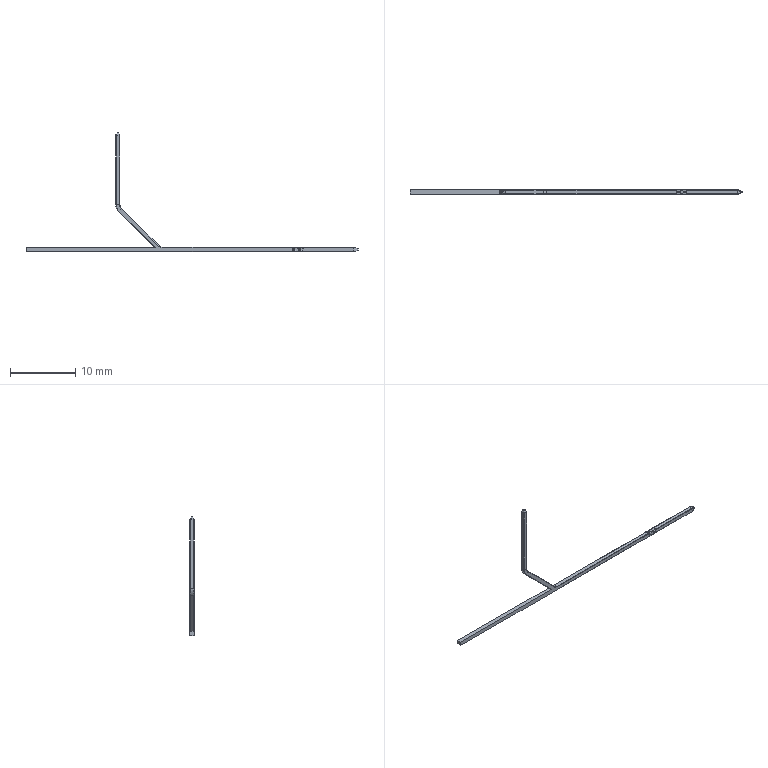Part | NX | features BREP 1 | 1 solid | 223 faces | box 51.03 x 0.8779 x 18.316 mm | volume 27.799 mm3 | cylinder 91 | plane 82 | torus 26 | sphere 20 | spline 4 | commonest cylinder face diameters 0.1 x32 0.09 x28 0.2 x12 2.01 x8 1 x4 2 x4